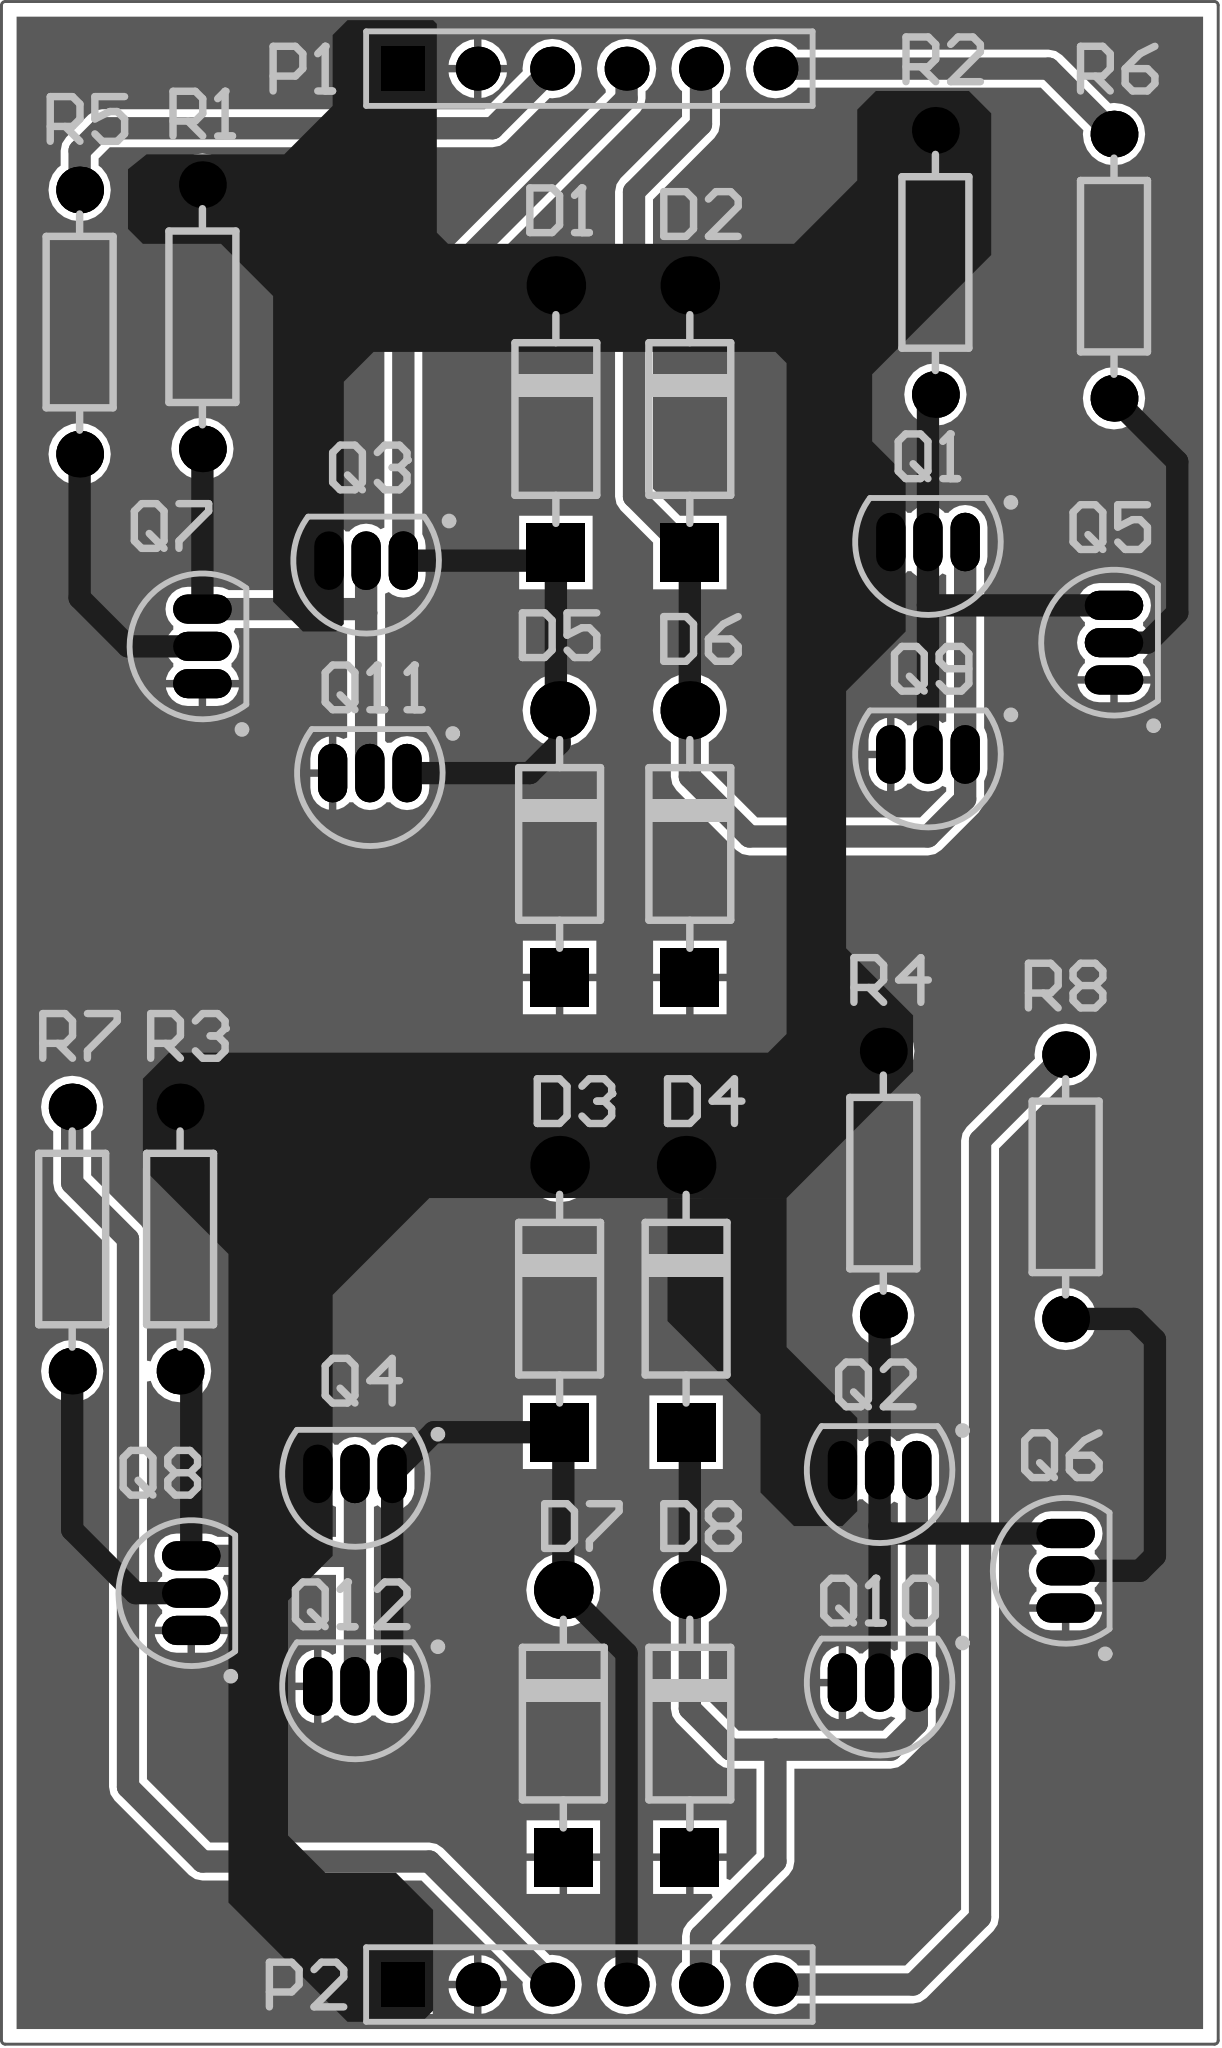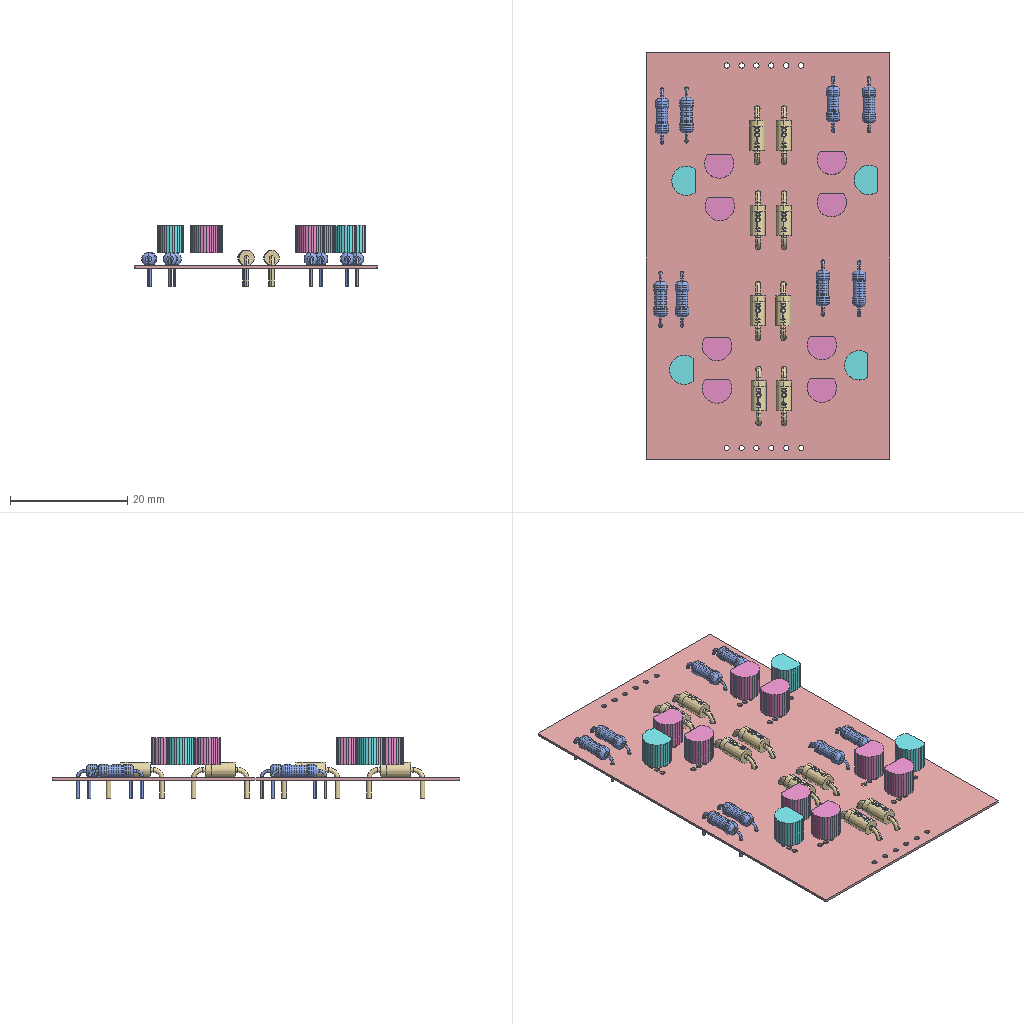Circuit board layout | Altium Designer | box 41.5 x 69.6 x 10.4 mm
Layer stack:
# Altium Designer layer stack of  (unit mm; dielectric type: 0 none, 1 core, 2 prepreg, 3 surface material)
index,name,kind,layer,copper_thickness_mm,dielectric_type,dielectric_thickness_mm,dielectric_material,dielectric_constant
0,Top Paste,other,,,,,,
1,Top Overlay,other,,,,,,
2,Top Solder,dielectric,,,3,0.0102,Solder Resist,3.5
3,Top Layer,copper,Top Layer,0.0356,,,,
4,Dielectric 1,dielectric,,,0,0.32,FR-4,4.8
5,Bottom Layer,copper,Bottom Layer,0.0356,,,,
6,Bottom Solder,dielectric,,,3,0.0102,Solder Resist,3.5
7,Bottom Overlay,other,,,,,,
8,Bottom Paste,other,,,,,,
# drill layer pairs: low layer,high layer
drill_pair,Top Layer,Bottom Layer
Part placement:
Designator,Comment,Layer,Footprint,Center-X(mm),Center-Y(mm),Rotation
R8,100,TopLayer,RS_1/4W,106.68,70.231,270
R7,100,TopLayer,RS_1/4W,72.771,68.453,90
R6,100,TopLayer,RS_1/4W,108.331,101.6,270
R5,100,TopLayer,RS_1/4W,73.025,99.695,90
R4,1K,TopLayer,RS_1/4W,100.457,70.358,90
R3,1K,TopLayer,RS_1/4W,76.454,68.453,90
R2,1K,TopLayer,RS_1/4W,102.235,101.727,90
R1,1K,TopLayer,RS_1/4W,77.216,99.877,90
Q12,2N3906,TopLayer,TO-92A,82.423,53.213,90
Q11,2N3906,TopLayer,TO-92A,82.931,84.328,90
Q10,2N3906,TopLayer,TO-92A,100.33,53.34,90
Q9,2N3906,TopLayer,TO-92A,101.981,84.963,90
Q8,2N3904,TopLayer,TO-92A,76.835,56.388,0
Q7,2N3904,TopLayer,TO-92A,77.216,88.646,0
Q6,2N3904,TopLayer,TO-92A,106.68,57.15,360
Q5,2N3904,TopLayer,TO-92A,108.331,88.773,360
Q4,2N3904,TopLayer,TO-92A,82.423,60.452,90
Q3,2N3904,TopLayer,TO-92A,82.804,91.567,90
Q2,2N3904,TopLayer,TO-92A,100.33,60.579,90
Q1,2N3904,TopLayer,TO-92A,101.981,92.202,90
P2,Header 6,TopLayer,HDR1X6,90.424,43.053,360
P1,Header 6,TopLayer,HDR1X6,90.424,108.331,360
D8,1N4148,TopLayer,DO-41,93.853,51.943,90
D7,1N4148,TopLayer,DO-41,89.535,51.943,90
D6,1N4148,TopLayer,DO-41,93.853,81.915,90
D5,1N4148,TopLayer,DO-41,89.408,81.915,90
D4,1N4148,TopLayer,DO-41,93.726,66.421,90
D3,1N4148,TopLayer,DO-41,89.408,66.421,90
D2,1N4148,TopLayer,DO-41,93.853,96.393,90
D1,1N4148,TopLayer,DO-41,89.281,96.393,90
Pad and via stacks:
# Altium Designer via and pad stacks of  (unit mm). Each distinct definition once, with the count of objects using it.
# via: kind,start_layer,end_layer,hole_mm,diameter_mm,mode(0 simple;1 top-mid-bottom;2 full stack),diameter_per_layer,count,example_net
# pad: kind,layer,hole_mm,hole_type(0 round;1 square;2 slot),plating,top_size,top_shape(1 round;2 rect;3 octagon;9 rounded rect),mid_size,bottom_size,mode,footprint,size_per_layer,count,example
pad,Multi-Layer,1,0,plated,2x2,1,2x2,2x2,0,DO-41,,8,D8.2
pad,Multi-Layer,1,0,plated,2x2,2,2x2,2x2,0,DO-41,,8,D8.1
pad,Multi-Layer,0.9,0,plated,1.5x1.5,2,1.5x1.5,1.5x1.5,0,HDR1X6,,2,P2.1
pad,Multi-Layer,0.9,0,plated,1.5x1.5,1,1.5x1.5,1.5x1.5,0,HDR1X6,,10,P2.2
pad,Multi-Layer,0.6,0,plated,1.6x1.6,1,1.6x1.6,1.6x1.6,0,RS 1/4W,,16,R4.2
pad,Multi-Layer,0.9,0,plated,2x1,1,2x1,2x1,0,TO-92A,,36,Q2.3
Copper pours:
name,layer,net,type(0 solid;1 hatched;2 none)
D,Bottom Layer,GND,0
Design rules, without the lines most boards share:
# Altium Designer design rules of  (exported by Altium Designer, unit mm)
# columns: name | kind | enabled | priority | scope1 | scope2 | descriptor | typed fields (field=value)
SilkToSilkClearance | 55 | enabled | 1 | All | All | Silk to Silk (Clearance=0mil) (All),(All) |
SilkToSolderMaskClearance | 54 | enabled | 1 | IsPad | All | Silk To Solder Mask (Clearance=0mil) (IsPad),(All) |
MinimumSolderMaskSliver | 53 | enabled | 1 | All | All | Minimum Solder Mask Sliver (Gap=0mil) (All),(All) |
HoleToHoleClearance | 52 | enabled | 1 | All | All | Hole To Hole Clearance (Gap=10mil) (All),(All) | gap=0.254
DiffPairsRouting | 51 | enabled | 1 | All | All | Differential Pairs Uncoupled Length using the Gap Constraints (Min=10mil) (Max=10mil) (Prefered=10mil)  and Width Constraints (Min=15mil) (Max=15mil) (Prefered=15mil) (All) |
SolderMaskExpansion | 13 | enabled | 1 | All | All | Solder Mask Expansion (Expansion =4mil) (All) | expansion=0.1016
PasteMaskExpansion | 14 | enabled | 1 | All | All | Paste Mask Expansion (Expansion =0mil) (All) | expansion=0
RoutingVias | 11 | enabled | 1 | All | All | Routing Via (MinHoleWidth=28mil) (MaxHoleWidth=28mil) (PreferredHoleWidth=28mil) (MinWidth=50mil) (MaxWidth=50mil) (PreferedWidth=50mil) (All) | via_min_hole=0.7112 via_max_hole=0.7112 via_preferred_diameter=1.27 via_preferred_hole=0.7112
Width | 2 | enabled | 1 | All | All | Width Constraint (Min=10mil) (Max=100mil) (Preferred=10mil) (All) |
PolygonConnect | 20 | enabled | 1 | All | All | Polygon Connect Rule(Relief Connect )(Conductor Width=10mil) (Relief Angle=90 Angle) (Entries=4) (Air Gap Width=10mil) (All),(All) | connect_style(0=relief,1=direct,2=none)=0 relief_conductor_width=0.254 relief_entries=4
PlaneConnect | 6 | enabled | 1 | All | All | Power Plane Connect Rule(Relief Connect )(Expansion=20mil) (Conductor Width=10mil) (Air Gap=10mil) (Entries=4) (All) | relief_conductor_width=0.254 relief_entries=4 relief_expansion=0.508
Clearance | 0 | enabled | 1 | All | All | Clearance Constraint (Gap=10mil) (All),(All) | gap=0.254
Classes set for this board:
# Altium Designer classes of  (member kind: 0 net, 1 component, 2 from-to, 3 pad, 4 layer, 5 differential pair, 6 design channel, 7 polygon, 8 structure, 9 xSignal)
# columns: class name | member kind | superclass | members
Sheet1 | 1 | no | D1; D2; D3; D4; D5; D6; D7; D8; P1; P2; Q1; Q2; Q3; Q4; Q5; Q6; Q7; Q8; Q9; Q10; Q11; Q12; R1; R2; R3; R4; R5; R6; R7; R8;